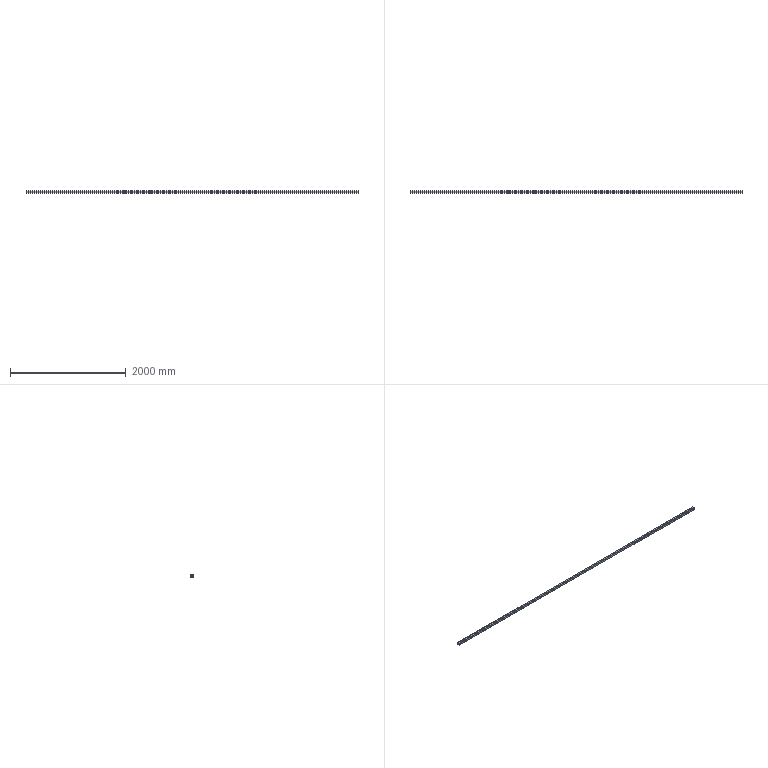Part | STEP file | SN10_003_008-04_TUBO_QUADRADO | 1 solid | 18 faces | box 5740 x 40 x 40 mm | volume 2415524 mm3 | plane 10 | cylinder 8 | commonest cylinder face diameters 6 x4 12 x4
STEP:
#1=CARTESIAN_POINT('',(0.,0.,0.));
#2=DIRECTION('',(0.,0.,1.));
#3=DIRECTION('',(1.,0.,0.));
#4=AXIS2_PLACEMENT_3D('',#1,#2,#3);
#5=CARTESIAN_POINT('',(0.,20.,14.));
#6=VERTEX_POINT('',#5);
#7=CARTESIAN_POINT('',(5740.,20.,14.));
#8=VERTEX_POINT('',#7);
#9=CARTESIAN_POINT('',(0.,20.,14.));
#10=DIRECTION('',(1.,0.,0.));
#11=VECTOR('',#10,1.);
#12=LINE('',#9,#11);
#13=CARTESIAN_POINT('',(2870.,14.,14.));
#14=DIRECTION('',(1.,0.,0.));
#15=DIRECTION('',(0.,1.,0.));
#16=AXIS2_PLACEMENT_3D('',#13,#14,#15);
#17=CYLINDRICAL_SURFACE('',#16,6.);
#18=CARTESIAN_POINT('',(0.,-2870.));
#19=DIRECTION('',(0.,1.));
#20=VECTOR('',#19,1.);
#21=LINE('',#18,#20);
#22=(GEOMETRIC_REPRESENTATION_CONTEXT(2)PARAMETRIC_REPRESENTATION_CONTEXT()REPRESENTATION_CONTEXT('',''));
#23=DEFINITIONAL_REPRESENTATION('',(#21),#22);
#24=PCURVE('',#17,#23);
#25=CARTESIAN_POINT('',(0.,20.,14.));
#26=DIRECTION('',(0.,-1.,0.));
#27=DIRECTION('',(0.,0.,-1.));
#28=AXIS2_PLACEMENT_3D('',#25,#26,#27);
#29=PLANE('',#28);
#30=CARTESIAN_POINT('',(0.,0.));
#31=DIRECTION('',(0.,1.));
#32=VECTOR('',#31,1.);
#33=LINE('',#30,#32);
#34=(GEOMETRIC_REPRESENTATION_CONTEXT(2)PARAMETRIC_REPRESENTATION_CONTEXT()REPRESENTATION_CONTEXT('',''));
#35=DEFINITIONAL_REPRESENTATION('',(#33),#34);
#36=PCURVE('',#29,#35);
#37=SURFACE_CURVE('',#12,(#24,#36),.PCURVE_S1.);
#38=EDGE_CURVE('',#6,#8,#37,.T.);
#39=ORIENTED_EDGE('',*,*,#38,.F.);
#40=CARTESIAN_POINT('',(0.,14.,20.));
#41=VERTEX_POINT('',#40);
#42=CARTESIAN_POINT('',(0.,14.,14.));
#43=DIRECTION('',(1.,0.,0.));
#44=DIRECTION('',(0.,1.,0.));
#45=AXIS2_PLACEMENT_3D('',#42,#43,#44);
#46=CIRCLE('',#45,6.);
#47=CARTESIAN_POINT('',(0.,-2870.));
#48=DIRECTION('',(1.,0.));
#49=VECTOR('',#48,1.);
#50=LINE('',#47,#49);
#51=(GEOMETRIC_REPRESENTATION_CONTEXT(2)PARAMETRIC_REPRESENTATION_CONTEXT()REPRESENTATION_CONTEXT('',''));
#52=DEFINITIONAL_REPRESENTATION('',(#50),#51);
#53=PCURVE('',#17,#52);
#54=CARTESIAN_POINT('',(0.,0.,0.));
#55=DIRECTION('',(1.,0.,0.));
#56=DIRECTION('',(0.,0.,-1.));
#57=AXIS2_PLACEMENT_3D('',#54,#55,#56);
#58=PLANE('',#57);
#59=CARTESIAN_POINT('',(-14.,14.));
#60=DIRECTION('',(0.,1.));
#61=AXIS2_PLACEMENT_2D('',#59,#60);
#62=CIRCLE('',#61,6.);
#63=(GEOMETRIC_REPRESENTATION_CONTEXT(2)PARAMETRIC_REPRESENTATION_CONTEXT()REPRESENTATION_CONTEXT('',''));
#64=DEFINITIONAL_REPRESENTATION('',(#62),#63);
#65=PCURVE('',#58,#64);
#66=SURFACE_CURVE('',#46,(#53,#65),.PCURVE_S1.);
#67=EDGE_CURVE('',#6,#41,#66,.T.);
#68=ORIENTED_EDGE('',*,*,#67,.T.);
#69=CARTESIAN_POINT('',(5740.,14.,20.));
#70=VERTEX_POINT('',#69);
#71=CARTESIAN_POINT('',(0.,14.,20.));
#72=DIRECTION('',(1.,0.,0.));
#73=VECTOR('',#72,1.);
#74=LINE('',#71,#73);
#75=CARTESIAN_POINT('',(1.571,-2870.));
#76=DIRECTION('',(0.,1.));
#77=VECTOR('',#76,1.);
#78=LINE('',#75,#77);
#79=(GEOMETRIC_REPRESENTATION_CONTEXT(2)PARAMETRIC_REPRESENTATION_CONTEXT()REPRESENTATION_CONTEXT('',''));
#80=DEFINITIONAL_REPRESENTATION('',(#78),#79);
#81=PCURVE('',#17,#80);
#82=CARTESIAN_POINT('',(0.,-14.,20.));
#83=DIRECTION('',(0.,0.,-1.));
#84=DIRECTION('',(-1.,0.,0.));
#85=AXIS2_PLACEMENT_3D('',#82,#83,#84);
#86=PLANE('',#85);
#87=CARTESIAN_POINT('',(0.,28.));
#88=DIRECTION('',(-1.,0.));
#89=VECTOR('',#88,1.);
#90=LINE('',#87,#89);
#91=(GEOMETRIC_REPRESENTATION_CONTEXT(2)PARAMETRIC_REPRESENTATION_CONTEXT()REPRESENTATION_CONTEXT('',''));
#92=DEFINITIONAL_REPRESENTATION('',(#90),#91);
#93=PCURVE('',#86,#92);
#94=SURFACE_CURVE('',#74,(#81,#93),.PCURVE_S1.);
#95=EDGE_CURVE('',#41,#70,#94,.T.);
#96=ORIENTED_EDGE('',*,*,#95,.T.);
#97=CARTESIAN_POINT('',(5740.,14.,14.));
#98=DIRECTION('',(1.,0.,0.));
#99=DIRECTION('',(0.,1.,0.));
#100=AXIS2_PLACEMENT_3D('',#97,#98,#99);
#101=CIRCLE('',#100,6.);
#102=CARTESIAN_POINT('',(0.,2870.));
#103=DIRECTION('',(1.,0.));
#104=VECTOR('',#103,1.);
#105=LINE('',#102,#104);
#106=(GEOMETRIC_REPRESENTATION_CONTEXT(2)PARAMETRIC_REPRESENTATION_CONTEXT()REPRESENTATION_CONTEXT('',''));
#107=DEFINITIONAL_REPRESENTATION('',(#105),#106);
#108=PCURVE('',#17,#107);
#109=CARTESIAN_POINT('',(5740.,0.,0.));
#110=DIRECTION('',(1.,0.,0.));
#111=DIRECTION('',(0.,0.,-1.));
#112=AXIS2_PLACEMENT_3D('',#109,#110,#111);
#113=PLANE('',#112);
#114=CARTESIAN_POINT('',(-14.,14.));
#115=DIRECTION('',(0.,1.));
#116=AXIS2_PLACEMENT_2D('',#114,#115);
#117=CIRCLE('',#116,6.);
#118=(GEOMETRIC_REPRESENTATION_CONTEXT(2)PARAMETRIC_REPRESENTATION_CONTEXT()REPRESENTATION_CONTEXT('',''));
#119=DEFINITIONAL_REPRESENTATION('',(#117),#118);
#120=PCURVE('',#113,#119);
#121=SURFACE_CURVE('',#101,(#108,#120),.PCURVE_S1.);
#122=EDGE_CURVE('',#8,#70,#121,.T.);
#123=ORIENTED_EDGE('',*,*,#122,.F.);
#124=EDGE_LOOP('',(#39,#68,#96,#123));
#125=FACE_BOUND('',#124,.T.);
#126=ADVANCED_FACE('',(#125),#17,.T.);
#127=ORIENTED_EDGE('',*,*,#95,.F.);
#128=CARTESIAN_POINT('',(0.,-14.,20.));
#129=VERTEX_POINT('',#128);
#130=CARTESIAN_POINT('',(0.,-14.,20.));
#131=DIRECTION('',(0.,1.,0.));
#132=VECTOR('',#131,1.);
#133=LINE('',#130,#132);
#134=CARTESIAN_POINT('',(0.,0.));
#135=DIRECTION('',(0.,1.));
#136=VECTOR('',#135,1.);
#137=LINE('',#134,#136);
#138=(GEOMETRIC_REPRESENTATION_CONTEXT(2)PARAMETRIC_REPRESENTATION_CONTEXT()REPRESENTATION_CONTEXT('',''));
#139=DEFINITIONAL_REPRESENTATION('',(#137),#138);
#140=PCURVE('',#86,#139);
#141=CARTESIAN_POINT('',(-20.,-14.));
#142=DIRECTION('',(0.,1.));
#143=VECTOR('',#142,1.);
#144=LINE('',#141,#143);
#145=(GEOMETRIC_REPRESENTATION_CONTEXT(2)PARAMETRIC_REPRESENTATION_CONTEXT()REPRESENTATION_CONTEXT('',''));
#146=DEFINITIONAL_REPRESENTATION('',(#144),#145);
#147=PCURVE('',#58,#146);
#148=SURFACE_CURVE('',#133,(#140,#147),.PCURVE_S1.);
#149=EDGE_CURVE('',#129,#41,#148,.T.);
#150=ORIENTED_EDGE('',*,*,#149,.F.);
#151=CARTESIAN_POINT('',(5740.,-14.,20.));
#152=VERTEX_POINT('',#151);
#153=CARTESIAN_POINT('',(0.,-14.,20.));
#154=DIRECTION('',(1.,0.,0.));
#155=VECTOR('',#154,1.);
#156=LINE('',#153,#155);
#157=CARTESIAN_POINT('',(0.,0.));
#158=DIRECTION('',(-1.,0.));
#159=VECTOR('',#158,1.);
#160=LINE('',#157,#159);
#161=(GEOMETRIC_REPRESENTATION_CONTEXT(2)PARAMETRIC_REPRESENTATION_CONTEXT()REPRESENTATION_CONTEXT('',''));
#162=DEFINITIONAL_REPRESENTATION('',(#160),#161);
#163=PCURVE('',#86,#162);
#164=CARTESIAN_POINT('',(2870.,-14.,14.));
#165=DIRECTION('',(1.,0.,0.));
#166=DIRECTION('',(0.,0.,1.));
#167=AXIS2_PLACEMENT_3D('',#164,#165,#166);
#168=CYLINDRICAL_SURFACE('',#167,6.);
#169=CARTESIAN_POINT('',(0.,-2870.));
#170=DIRECTION('',(0.,1.));
#171=VECTOR('',#170,1.);
#172=LINE('',#169,#171);
#173=(GEOMETRIC_REPRESENTATION_CONTEXT(2)PARAMETRIC_REPRESENTATION_CONTEXT()REPRESENTATION_CONTEXT('',''));
#174=DEFINITIONAL_REPRESENTATION('',(#172),#173);
#175=PCURVE('',#168,#174);
#176=SURFACE_CURVE('',#156,(#163,#175),.PCURVE_S1.);
#177=EDGE_CURVE('',#129,#152,#176,.T.);
#178=ORIENTED_EDGE('',*,*,#177,.T.);
#179=CARTESIAN_POINT('',(5740.,-14.,20.));
#180=DIRECTION('',(0.,1.,0.));
#181=VECTOR('',#180,1.);
#182=LINE('',#179,#181);
#183=CARTESIAN_POINT('',(-5740.,0.));
#184=DIRECTION('',(0.,1.));
#185=VECTOR('',#184,1.);
#186=LINE('',#183,#185);
#187=(GEOMETRIC_REPRESENTATION_CONTEXT(2)PARAMETRIC_REPRESENTATION_CONTEXT()REPRESENTATION_CONTEXT('',''));
#188=DEFINITIONAL_REPRESENTATION('',(#186),#187);
#189=PCURVE('',#86,#188);
#190=CARTESIAN_POINT('',(-20.,-14.));
#191=DIRECTION('',(0.,1.));
#192=VECTOR('',#191,1.);
#193=LINE('',#190,#192);
#194=(GEOMETRIC_REPRESENTATION_CONTEXT(2)PARAMETRIC_REPRESENTATION_CONTEXT()REPRESENTATION_CONTEXT('',''));
#195=DEFINITIONAL_REPRESENTATION('',(#193),#194);
#196=PCURVE('',#113,#195);
#197=SURFACE_CURVE('',#182,(#189,#196),.PCURVE_S1.);
#198=EDGE_CURVE('',#152,#70,#197,.T.);
#199=ORIENTED_EDGE('',*,*,#198,.T.);
#200=EDGE_LOOP('',(#127,#150,#178,#199));
#201=FACE_BOUND('',#200,.T.);
#202=ADVANCED_FACE('',(#201),#86,.F.);
#203=ORIENTED_EDGE('',*,*,#177,.F.);
#204=CARTESIAN_POINT('',(0.,-20.,14.));
#205=VERTEX_POINT('',#204);
#206=CARTESIAN_POINT('',(0.,-14.,14.));
#207=DIRECTION('',(1.,0.,0.));
#208=DIRECTION('',(0.,1.,0.));
#209=AXIS2_PLACEMENT_3D('',#206,#207,#208);
#210=CIRCLE('',#209,6.);
#211=CARTESIAN_POINT('',(-1.571,-2870.));
#212=DIRECTION('',(1.,0.));
#213=VECTOR('',#212,1.);
#214=LINE('',#211,#213);
#215=(GEOMETRIC_REPRESENTATION_CONTEXT(2)PARAMETRIC_REPRESENTATION_CONTEXT()REPRESENTATION_CONTEXT('',''));
#216=DEFINITIONAL_REPRESENTATION('',(#214),#215);
#217=PCURVE('',#168,#216);
#218=CARTESIAN_POINT('',(-14.,-14.));
#219=DIRECTION('',(0.,1.));
#220=AXIS2_PLACEMENT_2D('',#218,#219);
#221=CIRCLE('',#220,6.);
#222=(GEOMETRIC_REPRESENTATION_CONTEXT(2)PARAMETRIC_REPRESENTATION_CONTEXT()REPRESENTATION_CONTEXT('',''));
#223=DEFINITIONAL_REPRESENTATION('',(#221),#222);
#224=PCURVE('',#58,#223);
#225=SURFACE_CURVE('',#210,(#217,#224),.PCURVE_S1.);
#226=EDGE_CURVE('',#129,#205,#225,.T.);
#227=ORIENTED_EDGE('',*,*,#226,.T.);
#228=CARTESIAN_POINT('',(5740.,-20.,14.));
#229=VERTEX_POINT('',#228);
#230=CARTESIAN_POINT('',(0.,-20.,14.));
#231=DIRECTION('',(1.,0.,0.));
#232=VECTOR('',#231,1.);
#233=LINE('',#230,#232);
#234=CARTESIAN_POINT('',(1.571,-2870.));
#235=DIRECTION('',(0.,1.));
#236=VECTOR('',#235,1.);
#237=LINE('',#234,#236);
#238=(GEOMETRIC_REPRESENTATION_CONTEXT(2)PARAMETRIC_REPRESENTATION_CONTEXT()REPRESENTATION_CONTEXT('',''));
#239=DEFINITIONAL_REPRESENTATION('',(#237),#238);
#240=PCURVE('',#168,#239);
#241=CARTESIAN_POINT('',(0.,-20.,-14.));
#242=DIRECTION('',(0.,1.,0.));
#243=DIRECTION('',(0.,0.,1.));
#244=AXIS2_PLACEMENT_3D('',#241,#242,#243);
#245=PLANE('',#244);
#246=CARTESIAN_POINT('',(28.,0.));
#247=DIRECTION('',(0.,1.));
#248=VECTOR('',#247,1.);
#249=LINE('',#246,#248);
#250=(GEOMETRIC_REPRESENTATION_CONTEXT(2)PARAMETRIC_REPRESENTATION_CONTEXT()REPRESENTATION_CONTEXT('',''));
#251=DEFINITIONAL_REPRESENTATION('',(#249),#250);
#252=PCURVE('',#245,#251);
#253=SURFACE_CURVE('',#233,(#240,#252),.PCURVE_S1.);
#254=EDGE_CURVE('',#205,#229,#253,.T.);
#255=ORIENTED_EDGE('',*,*,#254,.T.);
#256=CARTESIAN_POINT('',(5740.,-14.,14.));
#257=DIRECTION('',(1.,0.,0.));
#258=DIRECTION('',(0.,1.,0.));
#259=AXIS2_PLACEMENT_3D('',#256,#257,#258);
#260=CIRCLE('',#259,6.);
#261=CARTESIAN_POINT('',(-1.571,2870.));
#262=DIRECTION('',(1.,0.));
#263=VECTOR('',#262,1.);
#264=LINE('',#261,#263);
#265=(GEOMETRIC_REPRESENTATION_CONTEXT(2)PARAMETRIC_REPRESENTATION_CONTEXT()REPRESENTATION_CONTEXT('',''));
#266=DEFINITIONAL_REPRESENTATION('',(#264),#265);
#267=PCURVE('',#168,#266);
#268=CARTESIAN_POINT('',(-14.,-14.));
#269=DIRECTION('',(0.,1.));
#270=AXIS2_PLACEMENT_2D('',#268,#269);
#271=CIRCLE('',#270,6.);
#272=(GEOMETRIC_REPRESENTATION_CONTEXT(2)PARAMETRIC_REPRESENTATION_CONTEXT()REPRESENTATION_CONTEXT('',''));
#273=DEFINITIONAL_REPRESENTATION('',(#271),#272);
#274=PCURVE('',#113,#273);
#275=SURFACE_CURVE('',#260,(#267,#274),.PCURVE_S1.);
#276=EDGE_CURVE('',#152,#229,#275,.T.);
#277=ORIENTED_EDGE('',*,*,#276,.F.);
#278=EDGE_LOOP('',(#203,#227,#255,#277));
#279=FACE_BOUND('',#278,.T.);
#280=ADVANCED_FACE('',(#279),#168,.T.);
#281=ORIENTED_EDGE('',*,*,#254,.F.);
#282=CARTESIAN_POINT('',(0.,-20.,-14.));
#283=VERTEX_POINT('',#282);
#284=CARTESIAN_POINT('',(0.,-20.,-14.));
#285=DIRECTION('',(0.,0.,1.));
#286=VECTOR('',#285,1.);
#287=LINE('',#284,#286);
#288=CARTESIAN_POINT('',(0.,0.));
#289=DIRECTION('',(1.,0.));
#290=VECTOR('',#289,1.);
#291=LINE('',#288,#290);
#292=(GEOMETRIC_REPRESENTATION_CONTEXT(2)PARAMETRIC_REPRESENTATION_CONTEXT()REPRESENTATION_CONTEXT('',''));
#293=DEFINITIONAL_REPRESENTATION('',(#291),#292);
#294=PCURVE('',#245,#293);
#295=CARTESIAN_POINT('',(14.,-20.));
#296=DIRECTION('',(-1.,0.));
#297=VECTOR('',#296,1.);
#298=LINE('',#295,#297);
#299=(GEOMETRIC_REPRESENTATION_CONTEXT(2)PARAMETRIC_REPRESENTATION_CONTEXT()REPRESENTATION_CONTEXT('',''));
#300=DEFINITIONAL_REPRESENTATION('',(#298),#299);
#301=PCURVE('',#58,#300);
#302=SURFACE_CURVE('',#287,(#294,#301),.PCURVE_S1.);
#303=EDGE_CURVE('',#283,#205,#302,.T.);
#304=ORIENTED_EDGE('',*,*,#303,.F.);
#305=CARTESIAN_POINT('',(5740.,-20.,-14.));
#306=VERTEX_POINT('',#305);
#307=CARTESIAN_POINT('',(0.,-20.,-14.));
#308=DIRECTION('',(1.,0.,0.));
#309=VECTOR('',#308,1.);
#310=LINE('',#307,#309);
#311=CARTESIAN_POINT('',(0.,0.));
#312=DIRECTION('',(0.,1.));
#313=VECTOR('',#312,1.);
#314=LINE('',#311,#313);
#315=(GEOMETRIC_REPRESENTATION_CONTEXT(2)PARAMETRIC_REPRESENTATION_CONTEXT()REPRESENTATION_CONTEXT('',''));
#316=DEFINITIONAL_REPRESENTATION('',(#314),#315);
#317=PCURVE('',#245,#316);
#318=CARTESIAN_POINT('',(2870.,-14.,-14.));
#319=DIRECTION('',(1.,0.,0.));
#320=DIRECTION('',(0.,-1.,0.));
#321=AXIS2_PLACEMENT_3D('',#318,#319,#320);
#322=CYLINDRICAL_SURFACE('',#321,6.);
#323=CARTESIAN_POINT('',(0.,-2870.));
#324=DIRECTION('',(0.,1.));
#325=VECTOR('',#324,1.);
#326=LINE('',#323,#325);
#327=(GEOMETRIC_REPRESENTATION_CONTEXT(2)PARAMETRIC_REPRESENTATION_CONTEXT()REPRESENTATION_CONTEXT('',''));
#328=DEFINITIONAL_REPRESENTATION('',(#326),#327);
#329=PCURVE('',#322,#328);
#330=SURFACE_CURVE('',#310,(#317,#329),.PCURVE_S1.);
#331=EDGE_CURVE('',#283,#306,#330,.T.);
#332=ORIENTED_EDGE('',*,*,#331,.T.);
#333=CARTESIAN_POINT('',(5740.,-20.,-14.));
#334=DIRECTION('',(0.,0.,1.));
#335=VECTOR('',#334,1.);
#336=LINE('',#333,#335);
#337=CARTESIAN_POINT('',(0.,5740.));
#338=DIRECTION('',(1.,0.));
#339=VECTOR('',#338,1.);
#340=LINE('',#337,#339);
#341=(GEOMETRIC_REPRESENTATION_CONTEXT(2)PARAMETRIC_REPRESENTATION_CONTEXT()REPRESENTATION_CONTEXT('',''));
#342=DEFINITIONAL_REPRESENTATION('',(#340),#341);
#343=PCURVE('',#245,#342);
#344=CARTESIAN_POINT('',(14.,-20.));
#345=DIRECTION('',(-1.,0.));
#346=VECTOR('',#345,1.);
#347=LINE('',#344,#346);
#348=(GEOMETRIC_REPRESENTATION_CONTEXT(2)PARAMETRIC_REPRESENTATION_CONTEXT()REPRESENTATION_CONTEXT('',''));
#349=DEFINITIONAL_REPRESENTATION('',(#347),#348);
#350=PCURVE('',#113,#349);
#351=SURFACE_CURVE('',#336,(#343,#350),.PCURVE_S1.);
#352=EDGE_CURVE('',#306,#229,#351,.T.);
#353=ORIENTED_EDGE('',*,*,#352,.T.);
#354=EDGE_LOOP('',(#281,#304,#332,#353));
#355=FACE_BOUND('',#354,.T.);
#356=ADVANCED_FACE('',(#355),#245,.F.);
#357=ORIENTED_EDGE('',*,*,#331,.F.);
#358=CARTESIAN_POINT('',(0.,-14.,-20.));
#359=VERTEX_POINT('',#358);
#360=CARTESIAN_POINT('',(0.,-14.,-14.));
#361=DIRECTION('',(1.,0.,0.));
#362=DIRECTION('',(0.,1.,0.));
#363=AXIS2_PLACEMENT_3D('',#360,#361,#362);
#364=CIRCLE('',#363,6.);
#365=CARTESIAN_POINT('',(-3.142,-2870.));
#366=DIRECTION('',(1.,0.));
#367=VECTOR('',#366,1.);
#368=LINE('',#365,#367);
#369=(GEOMETRIC_REPRESENTATION_CONTEXT(2)PARAMETRIC_REPRESENTATION_CONTEXT()REPRESENTATION_CONTEXT('',''));
#370=DEFINITIONAL_REPRESENTATION('',(#368),#369);
#371=PCURVE('',#322,#370);
#372=CARTESIAN_POINT('',(14.,-14.));
#373=DIRECTION('',(0.,1.));
#374=AXIS2_PLACEMENT_2D('',#372,#373);
#375=CIRCLE('',#374,6.);
#376=(GEOMETRIC_REPRESENTATION_CONTEXT(2)PARAMETRIC_REPRESENTATION_CONTEXT()REPRESENTATION_CONTEXT('',''));
#377=DEFINITIONAL_REPRESENTATION('',(#375),#376);
#378=PCURVE('',#58,#377);
#379=SURFACE_CURVE('',#364,(#371,#378),.PCURVE_S1.);
#380=EDGE_CURVE('',#283,#359,#379,.T.);
#381=ORIENTED_EDGE('',*,*,#380,.T.);
#382=CARTESIAN_POINT('',(5740.,-14.,-20.));
#383=VERTEX_POINT('',#382);
#384=CARTESIAN_POINT('',(0.,-14.,-20.));
#385=DIRECTION('',(1.,0.,0.));
#386=VECTOR('',#385,1.);
#387=LINE('',#384,#386);
#388=CARTESIAN_POINT('',(1.571,-2870.));
#389=DIRECTION('',(0.,1.));
#390=VECTOR('',#389,1.);
#391=LINE('',#388,#390);
#392=(GEOMETRIC_REPRESENTATION_CONTEXT(2)PARAMETRIC_REPRESENTATION_CONTEXT()REPRESENTATION_CONTEXT('',''));
#393=DEFINITIONAL_REPRESENTATION('',(#391),#392);
#394=PCURVE('',#322,#393);
#395=CARTESIAN_POINT('',(0.,14.,-20.));
#396=DIRECTION('',(0.,0.,1.));
#397=DIRECTION('',(1.,0.,0.));
#398=AXIS2_PLACEMENT_3D('',#395,#396,#397);
#399=PLANE('',#398);
#400=CARTESIAN_POINT('',(0.,-28.));
#401=DIRECTION('',(1.,0.));
#402=VECTOR('',#401,1.);
#403=LINE('',#400,#402);
#404=(GEOMETRIC_REPRESENTATION_CONTEXT(2)PARAMETRIC_REPRESENTATION_CONTEXT()REPRESENTATION_CONTEXT('',''));
#405=DEFINITIONAL_REPRESENTATION('',(#403),#404);
#406=PCURVE('',#399,#405);
#407=SURFACE_CURVE('',#387,(#394,#406),.PCURVE_S1.);
#408=EDGE_CURVE('',#359,#383,#407,.T.);
#409=ORIENTED_EDGE('',*,*,#408,.T.);
#410=CARTESIAN_POINT('',(5740.,-14.,-14.));
#411=DIRECTION('',(1.,0.,0.));
#412=DIRECTION('',(0.,1.,0.));
#413=AXIS2_PLACEMENT_3D('',#410,#411,#412);
#414=CIRCLE('',#413,6.);
#415=CARTESIAN_POINT('',(-3.142,2870.));
#416=DIRECTION('',(1.,0.));
#417=VECTOR('',#416,1.);
#418=LINE('',#415,#417);
#419=(GEOMETRIC_REPRESENTATION_CONTEXT(2)PARAMETRIC_REPRESENTATION_CONTEXT()REPRESENTATION_CONTEXT('',''));
#420=DEFINITIONAL_REPRESENTATION('',(#418),#419);
#421=PCURVE('',#322,#420);
#422=CARTESIAN_POINT('',(14.,-14.));
#423=DIRECTION('',(0.,1.));
#424=AXIS2_PLACEMENT_2D('',#422,#423);
#425=CIRCLE('',#424,6.);
#426=(GEOMETRIC_REPRESENTATION_CONTEXT(2)PARAMETRIC_REPRESENTATION_CONTEXT()REPRESENTATION_CONTEXT('',''));
#427=DEFINITIONAL_REPRESENTATION('',(#425),#426);
#428=PCURVE('',#113,#427);
#429=SURFACE_CURVE('',#414,(#421,#428),.PCURVE_S1.);
#430=EDGE_CURVE('',#306,#383,#429,.T.);
#431=ORIENTED_EDGE('',*,*,#430,.F.);
#432=EDGE_LOOP('',(#357,#381,#409,#431));
#433=FACE_BOUND('',#432,.T.);
#434=ADVANCED_FACE('',(#433),#322,.T.);
#435=ORIENTED_EDGE('',*,*,#408,.F.);
#436=CARTESIAN_POINT('',(0.,14.,-20.));
#437=VERTEX_POINT('',#436);
#438=CARTESIAN_POINT('',(0.,14.,-20.));
#439=DIRECTION('',(0.,-1.,0.));
#440=VECTOR('',#439,1.);
#441=LINE('',#438,#440);
#442=CARTESIAN_POINT('',(0.,0.));
#443=DIRECTION('',(0.,-1.));
#444=VECTOR('',#443,1.);
#445=LINE('',#442,#444);
#446=(GEOMETRIC_REPRESENTATION_CONTEXT(2)PARAMETRIC_REPRESENTATION_CONTEXT()REPRESENTATION_CONTEXT('',''));
#447=DEFINITIONAL_REPRESENTATION('',(#445),#446);
#448=PCURVE('',#399,#447);
#449=CARTESIAN_POINT('',(20.,14.));
#450=DIRECTION('',(0.,-1.));
#451=VECTOR('',#450,1.);
#452=LINE('',#449,#451);
#453=(GEOMETRIC_REPRESENTATION_CONTEXT(2)PARAMETRIC_REPRESENTATION_CONTEXT()REPRESENTATION_CONTEXT('',''));
#454=DEFINITIONAL_REPRESENTATION('',(#452),#453);
#455=PCURVE('',#58,#454);
#456=SURFACE_CURVE('',#441,(#448,#455),.PCURVE_S1.);
#457=EDGE_CURVE('',#437,#359,#456,.T.);
#458=ORIENTED_EDGE('',*,*,#457,.F.);
#459=CARTESIAN_POINT('',(5740.,14.,-20.));
#460=VERTEX_POINT('',#459);
#461=CARTESIAN_POINT('',(0.,14.,-20.));
#462=DIRECTION('',(1.,0.,0.));
#463=VECTOR('',#462,1.);
#464=LINE('',#461,#463);
#465=CARTESIAN_POINT('',(0.,0.));
#466=DIRECTION('',(1.,0.));
#467=VECTOR('',#466,1.);
#468=LINE('',#465,#467);
#469=(GEOMETRIC_REPRESENTATION_CONTEXT(2)PARAMETRIC_REPRESENTATION_CONTEXT()REPRESENTATION_CONTEXT('',''));
#470=DEFINITIONAL_REPRESENTATION('',(#468),#469);
#471=PCURVE('',#399,#470);
#472=CARTESIAN_POINT('',(2870.,14.,-14.));
#473=DIRECTION('',(1.,0.,0.));
#474=DIRECTION('',(0.,0.,-1.));
#475=AXIS2_PLACEMENT_3D('',#472,#473,#474);
#476=CYLINDRICAL_SURFACE('',#475,6.);
#477=CARTESIAN_POINT('',(0.,-2870.));
#478=DIRECTION('',(0.,1.));
#479=VECTOR('',#478,1.);
#480=LINE('',#477,#479);
#481=(GEOMETRIC_REPRESENTATION_CONTEXT(2)PARAMETRIC_REPRESENTATION_CONTEXT()REPRESENTATION_CONTEXT('',''));
#482=DEFINITIONAL_REPRESENTATION('',(#480),#481);
#483=PCURVE('',#476,#482);
#484=SURFACE_CURVE('',#464,(#471,#483),.PCURVE_S1.);
#485=EDGE_CURVE('',#437,#460,#484,.T.);
#486=ORIENTED_EDGE('',*,*,#485,.T.);
#487=CARTESIAN_POINT('',(5740.,14.,-20.));
#488=DIRECTION('',(0.,-1.,0.));
#489=VECTOR('',#488,1.);
#490=LINE('',#487,#489);
#491=CARTESIAN_POINT('',(5740.,0.));
#492=DIRECTION('',(0.,-1.));
#493=VECTOR('',#492,1.);
#494=LINE('',#491,#493);
#495=(GEOMETRIC_REPRESENTATION_CONTEXT(2)PARAMETRIC_REPRESENTATION_CONTEXT()REPRESENTATION_CONTEXT('',''));
#496=DEFINITIONAL_REPRESENTATION('',(#494),#495);
#497=PCURVE('',#399,#496);
#498=CARTESIAN_POINT('',(20.,14.));
#499=DIRECTION('',(0.,-1.));
#500=VECTOR('',#499,1.);
#501=LINE('',#498,#500);
#502=(GEOMETRIC_REPRESENTATION_CONTEXT(2)PARAMETRIC_REPRESENTATION_CONTEXT()REPRESENTATION_CONTEXT('',''));
#503=DEFINITIONAL_REPRESENTATION('',(#501),#502);
#504=PCURVE('',#113,#503);
#505=SURFACE_CURVE('',#490,(#497,#504),.PCURVE_S1.);
#506=EDGE_CURVE('',#460,#383,#505,.T.);
#507=ORIENTED_EDGE('',*,*,#506,.T.);
#508=EDGE_LOOP('',(#435,#458,#486,#507));
#509=FACE_BOUND('',#508,.T.);
#510=ADVANCED_FACE('',(#509),#399,.F.);
#511=ORIENTED_EDGE('',*,*,#485,.F.);
#512=CARTESIAN_POINT('',(0.,20.,-14.));
#513=VERTEX_POINT('',#512);
#514=CARTESIAN_POINT('',(0.,14.,-14.));
#515=DIRECTION('',(1.,0.,0.));
#516=DIRECTION('',(0.,1.,0.));
#517=AXIS2_PLACEMENT_3D('',#514,#515,#516);
#518=CIRCLE('',#517,6.);
#519=CARTESIAN_POINT('',(-4.712,-2870.));
#520=DIRECTION('',(1.,0.));
#521=VECTOR('',#520,1.);
#522=LINE('',#519,#521);
#523=(GEOMETRIC_REPRESENTATION_CONTEXT(2)PARAMETRIC_REPRESENTATION_CONTEXT()REPRESENTATION_CONTEXT('',''));
#524=DEFINITIONAL_REPRESENTATION('',(#522),#523);
#525=PCURVE('',#476,#524);
#526=CARTESIAN_POINT('',(14.,14.));
#527=DIRECTION('',(0.,1.));
#528=AXIS2_PLACEMENT_2D('',#526,#527);
#529=CIRCLE('',#528,6.);
#530=(GEOMETRIC_REPRESENTATION_CONTEXT(2)PARAMETRIC_REPRESENTATION_CONTEXT()REPRESENTATION_CONTEXT('',''));
#531=DEFINITIONAL_REPRESENTATION('',(#529),#530);
#532=PCURVE('',#58,#531);
#533=SURFACE_CURVE('',#518,(#525,#532),.PCURVE_S1.);
#534=EDGE_CURVE('',#437,#513,#533,.T.);
#535=ORIENTED_EDGE('',*,*,#534,.T.);
#536=CARTESIAN_POINT('',(5740.,20.,-14.));
#537=VERTEX_POINT('',#536);
#538=CARTESIAN_POINT('',(0.,20.,-14.));
#539=DIRECTION('',(1.,0.,0.));
#540=VECTOR('',#539,1.);
#541=LINE('',#538,#540);
#542=CARTESIAN_POINT('',(1.571,-2870.));
#543=DIRECTION('',(0.,1.));
#544=VECTOR('',#543,1.);
#545=LINE('',#542,#544);
#546=(GEOMETRIC_REPRESENTATION_CONTEXT(2)PARAMETRIC_REPRESENTATION_CONTEXT()REPRESENTATION_CONTEXT('',''));
#547=DEFINITIONAL_REPRESENTATION('',(#545),#546);
#548=PCURVE('',#476,#547);
#549=CARTESIAN_POINT('',(28.,0.));
#550=DIRECTION('',(0.,1.));
#551=VECTOR('',#550,1.);
#552=LINE('',#549,#551);
#553=(GEOMETRIC_REPRESENTATION_CONTEXT(2)PARAMETRIC_REPRESENTATION_CONTEXT()REPRESENTATION_CONTEXT('',''));
#554=DEFINITIONAL_REPRESENTATION('',(#552),#553);
#555=PCURVE('',#29,#554);
#556=SURFACE_CURVE('',#541,(#548,#555),.PCURVE_S1.);
#557=EDGE_CURVE('',#513,#537,#556,.T.);
#558=ORIENTED_EDGE('',*,*,#557,.T.);
#559=CARTESIAN_POINT('',(5740.,14.,-14.));
#560=DIRECTION('',(1.,0.,0.));
#561=DIRECTION('',(0.,1.,0.));
#562=AXIS2_PLACEMENT_3D('',#559,#560,#561);
#563=CIRCLE('',#562,6.);
#564=CARTESIAN_POINT('',(-4.712,2870.));
#565=DIRECTION('',(1.,0.));
#566=VECTOR('',#565,1.);
#567=LINE('',#564,#566);
#568=(GEOMETRIC_REPRESENTATION_CONTEXT(2)PARAMETRIC_REPRESENTATION_CONTEXT()REPRESENTATION_CONTEXT('',''));
#569=DEFINITIONAL_REPRESENTATION('',(#567),#568);
#570=PCURVE('',#476,#569);
#571=CARTESIAN_POINT('',(14.,14.));
#572=DIRECTION('',(0.,1.));
#573=AXIS2_PLACEMENT_2D('',#571,#572);
#574=CIRCLE('',#573,6.);
#575=(GEOMETRIC_REPRESENTATION_CONTEXT(2)PARAMETRIC_REPRESENTATION_CONTEXT()REPRESENTATION_CONTEXT('',''));
#576=DEFINITIONAL_REPRESENTATION('',(#574),#575);
#577=PCURVE('',#113,#576);
#578=SURFACE_CURVE('',#563,(#570,#577),.PCURVE_S1.);
#579=EDGE_CURVE('',#460,#537,#578,.T.);
#580=ORIENTED_EDGE('',*,*,#579,.F.);
#581=EDGE_LOOP('',(#511,#535,#558,#580));
#582=FACE_BOUND('',#581,.T.);
#583=ADVANCED_FACE('',(#582),#476,.T.);
#584=ORIENTED_EDGE('',*,*,#557,.F.);
#585=CARTESIAN_POINT('',(0.,20.,14.));
#586=DIRECTION('',(0.,0.,-1.));
#587=VECTOR('',#586,1.);
#588=LINE('',#585,#587);
#589=CARTESIAN_POINT('',(0.,0.));
#590=DIRECTION('',(1.,0.));
#591=VECTOR('',#590,1.);
#592=LINE('',#589,#591);
#593=(GEOMETRIC_REPRESENTATION_CONTEXT(2)PARAMETRIC_REPRESENTATION_CONTEXT()REPRESENTATION_CONTEXT('',''));
#594=DEFINITIONAL_REPRESENTATION('',(#592),#593);
#595=PCURVE('',#29,#594);
#596=CARTESIAN_POINT('',(-14.,20.));
#597=DIRECTION('',(1.,0.));
#598=VECTOR('',#597,1.);
#599=LINE('',#596,#598);
#600=(GEOMETRIC_REPRESENTATION_CONTEXT(2)PARAMETRIC_REPRESENTATION_CONTEXT()REPRESENTATION_CONTEXT('',''));
#601=DEFINITIONAL_REPRESENTATION('',(#599),#600);
#602=PCURVE('',#58,#601);
#603=SURFACE_CURVE('',#588,(#595,#602),.PCURVE_S1.);
#604=EDGE_CURVE('',#6,#513,#603,.T.);
#605=ORIENTED_EDGE('',*,*,#604,.F.);
#606=ORIENTED_EDGE('',*,*,#38,.T.);
#607=CARTESIAN_POINT('',(5740.,20.,14.));
#608=DIRECTION('',(0.,0.,-1.));
#609=VECTOR('',#608,1.);
#610=LINE('',#607,#609);
#611=CARTESIAN_POINT('',(0.,5740.));
#612=DIRECTION('',(1.,0.));
#613=VECTOR('',#612,1.);
#614=LINE('',#611,#613);
#615=(GEOMETRIC_REPRESENTATION_CONTEXT(2)PARAMETRIC_REPRESENTATION_CONTEXT()REPRESENTATION_CONTEXT('',''));
#616=DEFINITIONAL_REPRESENTATION('',(#614),#615);
#617=PCURVE('',#29,#616);
#618=CARTESIAN_POINT('',(-14.,20.));
#619=DIRECTION('',(1.,0.));
#620=VECTOR('',#619,1.);
#621=LINE('',#618,#620);
#622=(GEOMETRIC_REPRESENTATION_CONTEXT(2)PARAMETRIC_REPRESENTATION_CONTEXT()REPRESENTATION_CONTEXT('',''));
#623=DEFINITIONAL_REPRESENTATION('',(#621),#622);
#624=PCURVE('',#113,#623);
#625=SURFACE_CURVE('',#610,(#617,#624),.PCURVE_S1.);
#626=EDGE_CURVE('',#8,#537,#625,.T.);
#627=ORIENTED_EDGE('',*,*,#626,.T.);
#628=EDGE_LOOP('',(#584,#605,#606,#627));
#629=FACE_BOUND('',#628,.T.);
#630=ADVANCED_FACE('',(#629),#29,.F.);
#631=CARTESIAN_POINT('',(5740.,17.,14.));
#632=VERTEX_POINT('',#631);
#633=CARTESIAN_POINT('',(5740.,17.,-14.));
#634=VERTEX_POINT('',#633);
#635=CARTESIAN_POINT('',(5740.,17.,14.));
#636=DIRECTION('',(0.,0.,-1.));
#637=VECTOR('',#636,1.);
#638=LINE('',#635,#637);
#639=CARTESIAN_POINT('',(0.,17.,14.));
#640=DIRECTION('',(0.,-1.,0.));
#641=DIRECTION('',(0.,0.,-1.));
#642=AXIS2_PLACEMENT_3D('',#639,#640,#641);
#643=PLANE('',#642);
#644=CARTESIAN_POINT('',(0.,5740.));
#645=DIRECTION('',(1.,0.));
#646=VECTOR('',#645,1.);
#647=LINE('',#644,#646);
#648=(GEOMETRIC_REPRESENTATION_CONTEXT(2)PARAMETRIC_REPRESENTATION_CONTEXT()REPRESENTATION_CONTEXT('',''));
#649=DEFINITIONAL_REPRESENTATION('',(#647),#648);
#650=PCURVE('',#643,#649);
#651=CARTESIAN_POINT('',(-14.,17.));
#652=DIRECTION('',(1.,0.));
#653=VECTOR('',#652,1.);
#654=LINE('',#651,#653);
#655=(GEOMETRIC_REPRESENTATION_CONTEXT(2)PARAMETRIC_REPRESENTATION_CONTEXT()REPRESENTATION_CONTEXT('',''));
#656=DEFINITIONAL_REPRESENTATION('',(#654),#655);
#657=PCURVE('',#113,#656);
#658=SURFACE_CURVE('',#638,(#650,#657),.PCURVE_S1.);
#659=EDGE_CURVE('',#632,#634,#658,.T.);
#660=ORIENTED_EDGE('',*,*,#659,.F.);
#661=CARTESIAN_POINT('',(0.,17.,14.));
#662=VERTEX_POINT('',#661);
#663=CARTESIAN_POINT('',(0.,17.,14.));
#664=DIRECTION('',(1.,0.,0.));
#665=VECTOR('',#664,1.);
#666=LINE('',#663,#665);
#667=CARTESIAN_POINT('',(0.,0.));
#668=DIRECTION('',(0.,1.));
#669=VECTOR('',#668,1.);
#670=LINE('',#667,#669);
#671=(GEOMETRIC_REPRESENTATION_CONTEXT(2)PARAMETRIC_REPRESENTATION_CONTEXT()REPRESENTATION_CONTEXT('',''));
#672=DEFINITIONAL_REPRESENTATION('',(#670),#671);
#673=PCURVE('',#643,#672);
#674=CARTESIAN_POINT('',(2870.,14.,14.));
#675=DIRECTION('',(1.,0.,0.));
#676=DIRECTION('',(0.,1.,0.));
#677=AXIS2_PLACEMENT_3D('',#674,#675,#676);
#678=CYLINDRICAL_SURFACE('',#677,3.);
#679=CARTESIAN_POINT('',(0.,-2870.));
#680=DIRECTION('',(0.,1.));
#681=VECTOR('',#680,1.);
#682=LINE('',#679,#681);
#683=(GEOMETRIC_REPRESENTATION_CONTEXT(2)PARAMETRIC_REPRESENTATION_CONTEXT()REPRESENTATION_CONTEXT('',''));
#684=DEFINITIONAL_REPRESENTATION('',(#682),#683);
#685=PCURVE('',#678,#684);
#686=SURFACE_CURVE('',#666,(#673,#685),.PCURVE_S1.);
#687=EDGE_CURVE('',#662,#632,#686,.T.);
#688=ORIENTED_EDGE('',*,*,#687,.F.);
#689=CARTESIAN_POINT('',(0.,17.,-14.));
#690=VERTEX_POINT('',#689);
#691=CARTESIAN_POINT('',(0.,17.,14.));
#692=DIRECTION('',(0.,0.,-1.));
#693=VECTOR('',#692,1.);
#694=LINE('',#691,#693);
#695=CARTESIAN_POINT('',(0.,0.));
#696=DIRECTION('',(1.,0.));
#697=VECTOR('',#696,1.);
#698=LINE('',#695,#697);
#699=(GEOMETRIC_REPRESENTATION_CONTEXT(2)PARAMETRIC_REPRESENTATION_CONTEXT()REPRESENTATION_CONTEXT('',''));
#700=DEFINITIONAL_REPRESENTATION('',(#698),#699);
#701=PCURVE('',#643,#700);
#702=CARTESIAN_POINT('',(-14.,17.));
#703=DIRECTION('',(1.,0.));
#704=VECTOR('',#703,1.);
#705=LINE('',#702,#704);
#706=(GEOMETRIC_REPRESENTATION_CONTEXT(2)PARAMETRIC_REPRESENTATION_CONTEXT()REPRESENTATION_CONTEXT('',''));
#707=DEFINITIONAL_REPRESENTATION('',(#705),#706);
#708=PCURVE('',#58,#707);
#709=SURFACE_CURVE('',#694,(#701,#708),.PCURVE_S1.);
#710=EDGE_CURVE('',#662,#690,#709,.T.);
#711=ORIENTED_EDGE('',*,*,#710,.T.);
#712=CARTESIAN_POINT('',(0.,17.,-14.));
#713=DIRECTION('',(1.,0.,0.));
#714=VECTOR('',#713,1.);
#715=LINE('',#712,#714);
#716=CARTESIAN_POINT('',(28.,0.));
#717=DIRECTION('',(0.,1.));
#718=VECTOR('',#717,1.);
#719=LINE('',#716,#718);
#720=(GEOMETRIC_REPRESENTATION_CONTEXT(2)PARAMETRIC_REPRESENTATION_CONTEXT()REPRESENTATION_CONTEXT('',''));
#721=DEFINITIONAL_REPRESENTATION('',(#719),#720);
#722=PCURVE('',#643,#721);
#723=CARTESIAN_POINT('',(2870.,14.,-14.));
#724=DIRECTION('',(1.,0.,0.));
#725=DIRECTION('',(0.,0.,-1.));
#726=AXIS2_PLACEMENT_3D('',#723,#724,#725);
#727=CYLINDRICAL_SURFACE('',#726,3.);
#728=CARTESIAN_POINT('',(1.571,-2870.));
#729=DIRECTION('',(0.,1.));
#730=VECTOR('',#729,1.);
#731=LINE('',#728,#730);
#732=(GEOMETRIC_REPRESENTATION_CONTEXT(2)PARAMETRIC_REPRESENTATION_CONTEXT()REPRESENTATION_CONTEXT('',''));
#733=DEFINITIONAL_REPRESENTATION('',(#731),#732);
#734=PCURVE('',#727,#733);
#735=SURFACE_CURVE('',#715,(#722,#734),.PCURVE_S1.);
#736=EDGE_CURVE('',#690,#634,#735,.T.);
#737=ORIENTED_EDGE('',*,*,#736,.T.);
#738=EDGE_LOOP('',(#660,#688,#711,#737));
#739=FACE_BOUND('',#738,.T.);
#740=ADVANCED_FACE('',(#739),#643,.T.);
#741=CARTESIAN_POINT('',(0.,14.,-17.));
#742=VERTEX_POINT('',#741);
#743=CARTESIAN_POINT('',(5740.,14.,-17.));
#744=VERTEX_POINT('',#743);
#745=CARTESIAN_POINT('',(0.,14.,-17.));
#746=DIRECTION('',(1.,0.,0.));
#747=VECTOR('',#746,1.);
#748=LINE('',#745,#747);
#749=CARTESIAN_POINT('',(0.,-2870.));
#750=DIRECTION('',(0.,1.));
#751=VECTOR('',#750,1.);
#752=LINE('',#749,#751);
#753=(GEOMETRIC_REPRESENTATION_CONTEXT(2)PARAMETRIC_REPRESENTATION_CONTEXT()REPRESENTATION_CONTEXT('',''));
#754=DEFINITIONAL_REPRESENTATION('',(#752),#753);
#755=PCURVE('',#727,#754);
#756=CARTESIAN_POINT('',(0.,14.,-17.));
#757=DIRECTION('',(0.,0.,1.));
#758=DIRECTION('',(1.,0.,0.));
#759=AXIS2_PLACEMENT_3D('',#756,#757,#758);
#760=PLANE('',#759);
#761=CARTESIAN_POINT('',(0.,0.));
#762=DIRECTION('',(1.,0.));
#763=VECTOR('',#762,1.);
#764=LINE('',#761,#763);
#765=(GEOMETRIC_REPRESENTATION_CONTEXT(2)PARAMETRIC_REPRESENTATION_CONTEXT()REPRESENTATION_CONTEXT('',''));
#766=DEFINITIONAL_REPRESENTATION('',(#764),#765);
#767=PCURVE('',#760,#766);
#768=SURFACE_CURVE('',#748,(#755,#767),.PCURVE_S1.);
#769=EDGE_CURVE('',#742,#744,#768,.T.);
#770=ORIENTED_EDGE('',*,*,#769,.F.);
#771=CARTESIAN_POINT('',(0.,14.,-14.));
#772=DIRECTION('',(1.,0.,0.));
#773=DIRECTION('',(0.,1.,0.));
#774=AXIS2_PLACEMENT_3D('',#771,#772,#773);
#775=CIRCLE('',#774,3.);
#776=CARTESIAN_POINT('',(-4.712,-2870.));
#777=DIRECTION('',(1.,0.));
#778=VECTOR('',#777,1.);
#779=LINE('',#776,#778);
#780=(GEOMETRIC_REPRESENTATION_CONTEXT(2)PARAMETRIC_REPRESENTATION_CONTEXT()REPRESENTATION_CONTEXT('',''));
#781=DEFINITIONAL_REPRESENTATION('',(#779),#780);
#782=PCURVE('',#727,#781);
#783=CARTESIAN_POINT('',(14.,14.));
#784=DIRECTION('',(0.,1.));
#785=AXIS2_PLACEMENT_2D('',#783,#784);
#786=CIRCLE('',#785,3.);
#787=(GEOMETRIC_REPRESENTATION_CONTEXT(2)PARAMETRIC_REPRESENTATION_CONTEXT()REPRESENTATION_CONTEXT('',''));
#788=DEFINITIONAL_REPRESENTATION('',(#786),#787);
#789=PCURVE('',#58,#788);
#790=SURFACE_CURVE('',#775,(#782,#789),.PCURVE_S1.);
#791=EDGE_CURVE('',#742,#690,#790,.T.);
#792=ORIENTED_EDGE('',*,*,#791,.T.);
#793=ORIENTED_EDGE('',*,*,#736,.T.);
#794=CARTESIAN_POINT('',(5740.,14.,-14.));
#795=DIRECTION('',(1.,0.,0.));
#796=DIRECTION('',(0.,1.,0.));
#797=AXIS2_PLACEMENT_3D('',#794,#795,#796);
#798=CIRCLE('',#797,3.);
#799=CARTESIAN_POINT('',(-4.712,2870.));
#800=DIRECTION('',(1.,0.));
#801=VECTOR('',#800,1.);
#802=LINE('',#799,#801);
#803=(GEOMETRIC_REPRESENTATION_CONTEXT(2)PARAMETRIC_REPRESENTATION_CONTEXT()REPRESENTATION_CONTEXT('',''));
#804=DEFINITIONAL_REPRESENTATION('',(#802),#803);
#805=PCURVE('',#727,#804);
#806=CARTESIAN_POINT('',(14.,14.));
#807=DIRECTION('',(0.,1.));
#808=AXIS2_PLACEMENT_2D('',#806,#807);
#809=CIRCLE('',#808,3.);
#810=(GEOMETRIC_REPRESENTATION_CONTEXT(2)PARAMETRIC_REPRESENTATION_CONTEXT()REPRESENTATION_CONTEXT('',''));
#811=DEFINITIONAL_REPRESENTATION('',(#809),#810);
#812=PCURVE('',#113,#811);
#813=SURFACE_CURVE('',#798,(#805,#812),.PCURVE_S1.);
#814=EDGE_CURVE('',#744,#634,#813,.T.);
#815=ORIENTED_EDGE('',*,*,#814,.F.);
#816=EDGE_LOOP('',(#770,#792,#793,#815));
#817=FACE_BOUND('',#816,.F.);
#818=ADVANCED_FACE('',(#817),#727,.F.);
#819=CARTESIAN_POINT('',(5740.,-14.,-17.));
#820=VERTEX_POINT('',#819);
#821=CARTESIAN_POINT('',(5740.,14.,-17.));
#822=DIRECTION('',(0.,-1.,0.));
#823=VECTOR('',#822,1.);
#824=LINE('',#821,#823);
#825=CARTESIAN_POINT('',(5740.,0.));
#826=DIRECTION('',(0.,-1.));
#827=VECTOR('',#826,1.);
#828=LINE('',#825,#827);
#829=(GEOMETRIC_REPRESENTATION_CONTEXT(2)PARAMETRIC_REPRESENTATION_CONTEXT()REPRESENTATION_CONTEXT('',''));
#830=DEFINITIONAL_REPRESENTATION('',(#828),#829);
#831=PCURVE('',#760,#830);
#832=CARTESIAN_POINT('',(17.,14.));
#833=DIRECTION('',(0.,-1.));
#834=VECTOR('',#833,1.);
#835=LINE('',#832,#834);
#836=(GEOMETRIC_REPRESENTATION_CONTEXT(2)PARAMETRIC_REPRESENTATION_CONTEXT()REPRESENTATION_CONTEXT('',''));
#837=DEFINITIONAL_REPRESENTATION('',(#835),#836);
#838=PCURVE('',#113,#837);
#839=SURFACE_CURVE('',#824,(#831,#838),.PCURVE_S1.);
#840=EDGE_CURVE('',#744,#820,#839,.T.);
#841=ORIENTED_EDGE('',*,*,#840,.F.);
#842=ORIENTED_EDGE('',*,*,#769,.F.);
#843=CARTESIAN_POINT('',(0.,-14.,-17.));
#844=VERTEX_POINT('',#843);
#845=CARTESIAN_POINT('',(0.,14.,-17.));
#846=DIRECTION('',(0.,-1.,0.));
#847=VECTOR('',#846,1.);
#848=LINE('',#845,#847);
#849=CARTESIAN_POINT('',(0.,0.));
#850=DIRECTION('',(0.,-1.));
#851=VECTOR('',#850,1.);
#852=LINE('',#849,#851);
#853=(GEOMETRIC_REPRESENTATION_CONTEXT(2)PARAMETRIC_REPRESENTATION_CONTEXT()REPRESENTATION_CONTEXT('',''));
#854=DEFINITIONAL_REPRESENTATION('',(#852),#853);
#855=PCURVE('',#760,#854);
#856=CARTESIAN_POINT('',(17.,14.));
#857=DIRECTION('',(0.,-1.));
#858=VECTOR('',#857,1.);
#859=LINE('',#856,#858);
#860=(GEOMETRIC_REPRESENTATION_CONTEXT(2)PARAMETRIC_REPRESENTATION_CONTEXT()REPRESENTATION_CONTEXT('',''));
#861=DEFINITIONAL_REPRESENTATION('',(#859),#860);
#862=PCURVE('',#58,#861);
#863=SURFACE_CURVE('',#848,(#855,#862),.PCURVE_S1.);
#864=EDGE_CURVE('',#742,#844,#863,.T.);
#865=ORIENTED_EDGE('',*,*,#864,.T.);
#866=CARTESIAN_POINT('',(0.,-14.,-17.));
#867=DIRECTION('',(1.,0.,0.));
#868=VECTOR('',#867,1.);
#869=LINE('',#866,#868);
#870=CARTESIAN_POINT('',(0.,-28.));
#871=DIRECTION('',(1.,0.));
#872=VECTOR('',#871,1.);
#873=LINE('',#870,#872);
#874=(GEOMETRIC_REPRESENTATION_CONTEXT(2)PARAMETRIC_REPRESENTATION_CONTEXT()REPRESENTATION_CONTEXT('',''));
#875=DEFINITIONAL_REPRESENTATION('',(#873),#874);
#876=PCURVE('',#760,#875);
#877=CARTESIAN_POINT('',(2870.,-14.,-14.));
#878=DIRECTION('',(1.,0.,0.));
#879=DIRECTION('',(0.,-1.,0.));
#880=AXIS2_PLACEMENT_3D('',#877,#878,#879);
#881=CYLINDRICAL_SURFACE('',#880,3.);
#882=CARTESIAN_POINT('',(1.571,-2870.));
#883=DIRECTION('',(0.,1.));
#884=VECTOR('',#883,1.);
#885=LINE('',#882,#884);
#886=(GEOMETRIC_REPRESENTATION_CONTEXT(2)PARAMETRIC_REPRESENTATION_CONTEXT()REPRESENTATION_CONTEXT('',''));
#887=DEFINITIONAL_REPRESENTATION('',(#885),#886);
#888=PCURVE('',#881,#887);
#889=SURFACE_CURVE('',#869,(#876,#888),.PCURVE_S1.);
#890=EDGE_CURVE('',#844,#820,#889,.T.);
#891=ORIENTED_EDGE('',*,*,#890,.T.);
#892=EDGE_LOOP('',(#841,#842,#865,#891));
#893=FACE_BOUND('',#892,.T.);
#894=ADVANCED_FACE('',(#893),#760,.T.);
#895=CARTESIAN_POINT('',(0.,-17.,-14.));
#896=VERTEX_POINT('',#895);
#897=CARTESIAN_POINT('',(5740.,-17.,-14.));
#898=VERTEX_POINT('',#897);
#899=CARTESIAN_POINT('',(0.,-17.,-14.));
#900=DIRECTION('',(1.,0.,0.));
#901=VECTOR('',#900,1.);
#902=LINE('',#899,#901);
#903=CARTESIAN_POINT('',(0.,-2870.));
#904=DIRECTION('',(0.,1.));
#905=VECTOR('',#904,1.);
#906=LINE('',#903,#905);
#907=(GEOMETRIC_REPRESENTATION_CONTEXT(2)PARAMETRIC_REPRESENTATION_CONTEXT()REPRESENTATION_CONTEXT('',''));
#908=DEFINITIONAL_REPRESENTATION('',(#906),#907);
#909=PCURVE('',#881,#908);
#910=CARTESIAN_POINT('',(0.,-17.,-14.));
#911=DIRECTION('',(0.,1.,0.));
#912=DIRECTION('',(0.,0.,1.));
#913=AXIS2_PLACEMENT_3D('',#910,#911,#912);
#914=PLANE('',#913);
#915=CARTESIAN_POINT('',(0.,0.));
#916=DIRECTION('',(0.,1.));
#917=VECTOR('',#916,1.);
#918=LINE('',#915,#917);
#919=(GEOMETRIC_REPRESENTATION_CONTEXT(2)PARAMETRIC_REPRESENTATION_CONTEXT()REPRESENTATION_CONTEXT('',''));
#920=DEFINITIONAL_REPRESENTATION('',(#918),#919);
#921=PCURVE('',#914,#920);
#922=SURFACE_CURVE('',#902,(#909,#921),.PCURVE_S1.);
#923=EDGE_CURVE('',#896,#898,#922,.T.);
#924=ORIENTED_EDGE('',*,*,#923,.F.);
#925=CARTESIAN_POINT('',(0.,-14.,-14.));
#926=DIRECTION('',(1.,0.,0.));
#927=DIRECTION('',(0.,1.,0.));
#928=AXIS2_PLACEMENT_3D('',#925,#926,#927);
#929=CIRCLE('',#928,3.);
#930=CARTESIAN_POINT('',(-3.142,-2870.));
#931=DIRECTION('',(1.,0.));
#932=VECTOR('',#931,1.);
#933=LINE('',#930,#932);
#934=(GEOMETRIC_REPRESENTATION_CONTEXT(2)PARAMETRIC_REPRESENTATION_CONTEXT()REPRESENTATION_CONTEXT('',''));
#935=DEFINITIONAL_REPRESENTATION('',(#933),#934);
#936=PCURVE('',#881,#935);
#937=CARTESIAN_POINT('',(14.,-14.));
#938=DIRECTION('',(0.,1.));
#939=AXIS2_PLACEMENT_2D('',#937,#938);
#940=CIRCLE('',#939,3.);
#941=(GEOMETRIC_REPRESENTATION_CONTEXT(2)PARAMETRIC_REPRESENTATION_CONTEXT()REPRESENTATION_CONTEXT('',''));
#942=DEFINITIONAL_REPRESENTATION('',(#940),#941);
#943=PCURVE('',#58,#942);
#944=SURFACE_CURVE('',#929,(#936,#943),.PCURVE_S1.);
#945=EDGE_CURVE('',#896,#844,#944,.T.);
#946=ORIENTED_EDGE('',*,*,#945,.T.);
#947=ORIENTED_EDGE('',*,*,#890,.T.);
#948=CARTESIAN_POINT('',(5740.,-14.,-14.));
#949=DIRECTION('',(1.,0.,0.));
#950=DIRECTION('',(0.,1.,0.));
#951=AXIS2_PLACEMENT_3D('',#948,#949,#950);
#952=CIRCLE('',#951,3.);
#953=CARTESIAN_POINT('',(-3.142,2870.));
#954=DIRECTION('',(1.,0.));
#955=VECTOR('',#954,1.);
#956=LINE('',#953,#955);
#957=(GEOMETRIC_REPRESENTATION_CONTEXT(2)PARAMETRIC_REPRESENTATION_CONTEXT()REPRESENTATION_CONTEXT('',''));
#958=DEFINITIONAL_REPRESENTATION('',(#956),#957);
#959=PCURVE('',#881,#958);
#960=CARTESIAN_POINT('',(14.,-14.));
#961=DIRECTION('',(0.,1.));
#962=AXIS2_PLACEMENT_2D('',#960,#961);
#963=CIRCLE('',#962,3.);
#964=(GEOMETRIC_REPRESENTATION_CONTEXT(2)PARAMETRIC_REPRESENTATION_CONTEXT()REPRESENTATION_CONTEXT('',''));
#965=DEFINITIONAL_REPRESENTATION('',(#963),#964);
#966=PCURVE('',#113,#965);
#967=SURFACE_CURVE('',#952,(#959,#966),.PCURVE_S1.);
#968=EDGE_CURVE('',#898,#820,#967,.T.);
#969=ORIENTED_EDGE('',*,*,#968,.F.);
#970=EDGE_LOOP('',(#924,#946,#947,#969));
#971=FACE_BOUND('',#970,.F.);
#972=ADVANCED_FACE('',(#971),#881,.F.);
#973=CARTESIAN_POINT('',(5740.,-17.,14.));
#974=VERTEX_POINT('',#973);
#975=CARTESIAN_POINT('',(5740.,-17.,-14.));
#976=DIRECTION('',(0.,0.,1.));
#977=VECTOR('',#976,1.);
#978=LINE('',#975,#977);
#979=CARTESIAN_POINT('',(0.,5740.));
#980=DIRECTION('',(1.,0.));
#981=VECTOR('',#980,1.);
#982=LINE('',#979,#981);
#983=(GEOMETRIC_REPRESENTATION_CONTEXT(2)PARAMETRIC_REPRESENTATION_CONTEXT()REPRESENTATION_CONTEXT('',''));
#984=DEFINITIONAL_REPRESENTATION('',(#982),#983);
#985=PCURVE('',#914,#984);
#986=CARTESIAN_POINT('',(14.,-17.));
#987=DIRECTION('',(-1.,0.));
#988=VECTOR('',#987,1.);
#989=LINE('',#986,#988);
#990=(GEOMETRIC_REPRESENTATION_CONTEXT(2)PARAMETRIC_REPRESENTATION_CONTEXT()REPRESENTATION_CONTEXT('',''));
#991=DEFINITIONAL_REPRESENTATION('',(#989),#990);
#992=PCURVE('',#113,#991);
#993=SURFACE_CURVE('',#978,(#985,#992),.PCURVE_S1.);
#994=EDGE_CURVE('',#898,#974,#993,.T.);
#995=ORIENTED_EDGE('',*,*,#994,.F.);
#996=ORIENTED_EDGE('',*,*,#923,.F.);
#997=CARTESIAN_POINT('',(0.,-17.,14.));
#998=VERTEX_POINT('',#997);
#999=CARTESIAN_POINT('',(0.,-17.,-14.));
#1000=DIRECTION('',(0.,0.,1.));
#1001=VECTOR('',#1000,1.);
#1002=LINE('',#999,#1001);
#1003=CARTESIAN_POINT('',(0.,0.));
#1004=DIRECTION('',(1.,0.));
#1005=VECTOR('',#1004,1.);
#1006=LINE('',#1003,#1005);
#1007=(GEOMETRIC_REPRESENTATION_CONTEXT(2)PARAMETRIC_REPRESENTATION_CONTEXT()REPRESENTATION_CONTEXT('',''));
#1008=DEFINITIONAL_REPRESENTATION('',(#1006),#1007);
#1009=PCURVE('',#914,#1008);
#1010=CARTESIAN_POINT('',(14.,-17.));
#1011=DIRECTION('',(-1.,0.));
#1012=VECTOR('',#1011,1.);
#1013=LINE('',#1010,#1012);
#1014=(GEOMETRIC_REPRESENTATION_CONTEXT(2)PARAMETRIC_REPRESENTATION_CONTEXT()REPRESENTATION_CONTEXT('',''));
#1015=DEFINITIONAL_REPRESENTATION('',(#1013),#1014);
#1016=PCURVE('',#58,#1015);
#1017=SURFACE_CURVE('',#1002,(#1009,#1016),.PCURVE_S1.);
#1018=EDGE_CURVE('',#896,#998,#1017,.T.);
#1019=ORIENTED_EDGE('',*,*,#1018,.T.);
#1020=CARTESIAN_POINT('',(0.,-17.,14.));
#1021=DIRECTION('',(1.,0.,0.));
#1022=VECTOR('',#1021,1.);
#1023=LINE('',#1020,#1022);
#1024=CARTESIAN_POINT('',(28.,0.));
#1025=DIRECTION('',(0.,1.));
#1026=VECTOR('',#1025,1.);
#1027=LINE('',#1024,#1026);
#1028=(GEOMETRIC_REPRESENTATION_CONTEXT(2)PARAMETRIC_REPRESENTATION_CONTEXT()REPRESENTATION_CONTEXT('',''));
#1029=DEFINITIONAL_REPRESENTATION('',(#1027),#1028);
#1030=PCURVE('',#914,#1029);
#1031=CARTESIAN_POINT('',(2870.,-14.,14.));
#1032=DIRECTION('',(1.,0.,0.));
#1033=DIRECTION('',(0.,0.,1.));
#1034=AXIS2_PLACEMENT_3D('',#1031,#1032,#1033);
#1035=CYLINDRICAL_SURFACE('',#1034,3.);
#1036=CARTESIAN_POINT('',(1.571,-2870.));
#1037=DIRECTION('',(0.,1.));
#1038=VECTOR('',#1037,1.);
#1039=LINE('',#1036,#1038);
#1040=(GEOMETRIC_REPRESENTATION_CONTEXT(2)PARAMETRIC_REPRESENTATION_CONTEXT()REPRESENTATION_CONTEXT('',''));
#1041=DEFINITIONAL_REPRESENTATION('',(#1039),#1040);
#1042=PCURVE('',#1035,#1041);
#1043=SURFACE_CURVE('',#1023,(#1030,#1042),.PCURVE_S1.);
#1044=EDGE_CURVE('',#998,#974,#1043,.T.);
#1045=ORIENTED_EDGE('',*,*,#1044,.T.);
#1046=EDGE_LOOP('',(#995,#996,#1019,#1045));
#1047=FACE_BOUND('',#1046,.T.);
#1048=ADVANCED_FACE('',(#1047),#914,.T.);
#1049=CARTESIAN_POINT('',(0.,-14.,17.));
#1050=VERTEX_POINT('',#1049);
#1051=CARTESIAN_POINT('',(5740.,-14.,17.));
#1052=VERTEX_POINT('',#1051);
#1053=CARTESIAN_POINT('',(0.,-14.,17.));
#1054=DIRECTION('',(1.,0.,0.));
#1055=VECTOR('',#1054,1.);
#1056=LINE('',#1053,#1055);
#1057=CARTESIAN_POINT('',(0.,-2870.));
#1058=DIRECTION('',(0.,1.));
#1059=VECTOR('',#1058,1.);
#1060=LINE('',#1057,#1059);
#1061=(GEOMETRIC_REPRESENTATION_CONTEXT(2)PARAMETRIC_REPRESENTATION_CONTEXT()REPRESENTATION_CONTEXT('',''));
#1062=DEFINITIONAL_REPRESENTATION('',(#1060),#1061);
#1063=PCURVE('',#1035,#1062);
#1064=CARTESIAN_POINT('',(0.,-14.,17.));
#1065=DIRECTION('',(0.,0.,-1.));
#1066=DIRECTION('',(-1.,0.,0.));
#1067=AXIS2_PLACEMENT_3D('',#1064,#1065,#1066);
#1068=PLANE('',#1067);
#1069=CARTESIAN_POINT('',(0.,0.));
#1070=DIRECTION('',(-1.,0.));
#1071=VECTOR('',#1070,1.);
#1072=LINE('',#1069,#1071);
#1073=(GEOMETRIC_REPRESENTATION_CONTEXT(2)PARAMETRIC_REPRESENTATION_CONTEXT()REPRESENTATION_CONTEXT('',''));
#1074=DEFINITIONAL_REPRESENTATION('',(#1072),#1073);
#1075=PCURVE('',#1068,#1074);
#1076=SURFACE_CURVE('',#1056,(#1063,#1075),.PCURVE_S1.);
#1077=EDGE_CURVE('',#1050,#1052,#1076,.T.);
#1078=ORIENTED_EDGE('',*,*,#1077,.F.);
#1079=CARTESIAN_POINT('',(0.,-14.,14.));
#1080=DIRECTION('',(1.,0.,0.));
#1081=DIRECTION('',(0.,1.,0.));
#1082=AXIS2_PLACEMENT_3D('',#1079,#1080,#1081);
#1083=CIRCLE('',#1082,3.);
#1084=CARTESIAN_POINT('',(-1.571,-2870.));
#1085=DIRECTION('',(1.,0.));
#1086=VECTOR('',#1085,1.);
#1087=LINE('',#1084,#1086);
#1088=(GEOMETRIC_REPRESENTATION_CONTEXT(2)PARAMETRIC_REPRESENTATION_CONTEXT()REPRESENTATION_CONTEXT('',''));
#1089=DEFINITIONAL_REPRESENTATION('',(#1087),#1088);
#1090=PCURVE('',#1035,#1089);
#1091=CARTESIAN_POINT('',(-14.,-14.));
#1092=DIRECTION('',(0.,1.));
#1093=AXIS2_PLACEMENT_2D('',#1091,#1092);
#1094=CIRCLE('',#1093,3.);
#1095=(GEOMETRIC_REPRESENTATION_CONTEXT(2)PARAMETRIC_REPRESENTATION_CONTEXT()REPRESENTATION_CONTEXT('',''));
#1096=DEFINITIONAL_REPRESENTATION('',(#1094),#1095);
#1097=PCURVE('',#58,#1096);
#1098=SURFACE_CURVE('',#1083,(#1090,#1097),.PCURVE_S1.);
#1099=EDGE_CURVE('',#1050,#998,#1098,.T.);
#1100=ORIENTED_EDGE('',*,*,#1099,.T.);
#1101=ORIENTED_EDGE('',*,*,#1044,.T.);
#1102=CARTESIAN_POINT('',(5740.,-14.,14.));
#1103=DIRECTION('',(1.,0.,0.));
#1104=DIRECTION('',(0.,1.,0.));
#1105=AXIS2_PLACEMENT_3D('',#1102,#1103,#1104);
#1106=CIRCLE('',#1105,3.);
#1107=CARTESIAN_POINT('',(-1.571,2870.));
#1108=DIRECTION('',(1.,0.));
#1109=VECTOR('',#1108,1.);
#1110=LINE('',#1107,#1109);
#1111=(GEOMETRIC_REPRESENTATION_CONTEXT(2)PARAMETRIC_REPRESENTATION_CONTEXT()REPRESENTATION_CONTEXT('',''));
#1112=DEFINITIONAL_REPRESENTATION('',(#1110),#1111);
#1113=PCURVE('',#1035,#1112);
#1114=CARTESIAN_POINT('',(-14.,-14.));
#1115=DIRECTION('',(0.,1.));
#1116=AXIS2_PLACEMENT_2D('',#1114,#1115);
#1117=CIRCLE('',#1116,3.);
#1118=(GEOMETRIC_REPRESENTATION_CONTEXT(2)PARAMETRIC_REPRESENTATION_CONTEXT()REPRESENTATION_CONTEXT('',''));
#1119=DEFINITIONAL_REPRESENTATION('',(#1117),#1118);
#1120=PCURVE('',#113,#1119);
#1121=SURFACE_CURVE('',#1106,(#1113,#1120),.PCURVE_S1.);
#1122=EDGE_CURVE('',#1052,#974,#1121,.T.);
#1123=ORIENTED_EDGE('',*,*,#1122,.F.);
#1124=EDGE_LOOP('',(#1078,#1100,#1101,#1123));
#1125=FACE_BOUND('',#1124,.F.);
#1126=ADVANCED_FACE('',(#1125),#1035,.F.);
#1127=CARTESIAN_POINT('',(5740.,14.,17.));
#1128=VERTEX_POINT('',#1127);
#1129=CARTESIAN_POINT('',(5740.,-14.,17.));
#1130=DIRECTION('',(0.,1.,0.));
#1131=VECTOR('',#1130,1.);
#1132=LINE('',#1129,#1131);
#1133=CARTESIAN_POINT('',(-5740.,0.));
#1134=DIRECTION('',(0.,1.));
#1135=VECTOR('',#1134,1.);
#1136=LINE('',#1133,#1135);
#1137=(GEOMETRIC_REPRESENTATION_CONTEXT(2)PARAMETRIC_REPRESENTATION_CONTEXT()REPRESENTATION_CONTEXT('',''));
#1138=DEFINITIONAL_REPRESENTATION('',(#1136),#1137);
#1139=PCURVE('',#1068,#1138);
#1140=CARTESIAN_POINT('',(-17.,-14.));
#1141=DIRECTION('',(0.,1.));
#1142=VECTOR('',#1141,1.);
#1143=LINE('',#1140,#1142);
#1144=(GEOMETRIC_REPRESENTATION_CONTEXT(2)PARAMETRIC_REPRESENTATION_CONTEXT()REPRESENTATION_CONTEXT('',''));
#1145=DEFINITIONAL_REPRESENTATION('',(#1143),#1144);
#1146=PCURVE('',#113,#1145);
#1147=SURFACE_CURVE('',#1132,(#1139,#1146),.PCURVE_S1.);
#1148=EDGE_CURVE('',#1052,#1128,#1147,.T.);
#1149=ORIENTED_EDGE('',*,*,#1148,.F.);
#1150=ORIENTED_EDGE('',*,*,#1077,.F.);
#1151=CARTESIAN_POINT('',(0.,14.,17.));
#1152=VERTEX_POINT('',#1151);
#1153=CARTESIAN_POINT('',(0.,-14.,17.));
#1154=DIRECTION('',(0.,1.,0.));
#1155=VECTOR('',#1154,1.);
#1156=LINE('',#1153,#1155);
#1157=CARTESIAN_POINT('',(0.,0.));
#1158=DIRECTION('',(0.,1.));
#1159=VECTOR('',#1158,1.);
#1160=LINE('',#1157,#1159);
#1161=(GEOMETRIC_REPRESENTATION_CONTEXT(2)PARAMETRIC_REPRESENTATION_CONTEXT()REPRESENTATION_CONTEXT('',''));
#1162=DEFINITIONAL_REPRESENTATION('',(#1160),#1161);
#1163=PCURVE('',#1068,#1162);
#1164=CARTESIAN_POINT('',(-17.,-14.));
#1165=DIRECTION('',(0.,1.));
#1166=VECTOR('',#1165,1.);
#1167=LINE('',#1164,#1166);
#1168=(GEOMETRIC_REPRESENTATION_CONTEXT(2)PARAMETRIC_REPRESENTATION_CONTEXT()REPRESENTATION_CONTEXT('',''));
#1169=DEFINITIONAL_REPRESENTATION('',(#1167),#1168);
#1170=PCURVE('',#58,#1169);
#1171=SURFACE_CURVE('',#1156,(#1163,#1170),.PCURVE_S1.);
#1172=EDGE_CURVE('',#1050,#1152,#1171,.T.);
#1173=ORIENTED_EDGE('',*,*,#1172,.T.);
#1174=CARTESIAN_POINT('',(0.,14.,17.));
#1175=DIRECTION('',(1.,0.,0.));
#1176=VECTOR('',#1175,1.);
#1177=LINE('',#1174,#1176);
#1178=CARTESIAN_POINT('',(0.,28.));
#1179=DIRECTION('',(-1.,0.));
#1180=VECTOR('',#1179,1.);
#1181=LINE('',#1178,#1180);
#1182=(GEOMETRIC_REPRESENTATION_CONTEXT(2)PARAMETRIC_REPRESENTATION_CONTEXT()REPRESENTATION_CONTEXT('',''));
#1183=DEFINITIONAL_REPRESENTATION('',(#1181),#1182);
#1184=PCURVE('',#1068,#1183);
#1185=CARTESIAN_POINT('',(1.571,-2870.));
#1186=DIRECTION('',(0.,1.));
#1187=VECTOR('',#1186,1.);
#1188=LINE('',#1185,#1187);
#1189=(GEOMETRIC_REPRESENTATION_CONTEXT(2)PARAMETRIC_REPRESENTATION_CONTEXT()REPRESENTATION_CONTEXT('',''));
#1190=DEFINITIONAL_REPRESENTATION('',(#1188),#1189);
#1191=PCURVE('',#678,#1190);
#1192=SURFACE_CURVE('',#1177,(#1184,#1191),.PCURVE_S1.);
#1193=EDGE_CURVE('',#1152,#1128,#1192,.T.);
#1194=ORIENTED_EDGE('',*,*,#1193,.T.);
#1195=EDGE_LOOP('',(#1149,#1150,#1173,#1194));
#1196=FACE_BOUND('',#1195,.T.);
#1197=ADVANCED_FACE('',(#1196),#1068,.T.);
#1198=ORIENTED_EDGE('',*,*,#687,.F.);
#1199=CARTESIAN_POINT('',(0.,14.,14.));
#1200=DIRECTION('',(1.,0.,0.));
#1201=DIRECTION('',(0.,1.,0.));
#1202=AXIS2_PLACEMENT_3D('',#1199,#1200,#1201);
#1203=CIRCLE('',#1202,3.);
#1204=CARTESIAN_POINT('',(0.,-2870.));
#1205=DIRECTION('',(1.,0.));
#1206=VECTOR('',#1205,1.);
#1207=LINE('',#1204,#1206);
#1208=(GEOMETRIC_REPRESENTATION_CONTEXT(2)PARAMETRIC_REPRESENTATION_CONTEXT()REPRESENTATION_CONTEXT('',''));
#1209=DEFINITIONAL_REPRESENTATION('',(#1207),#1208);
#1210=PCURVE('',#678,#1209);
#1211=CARTESIAN_POINT('',(-14.,14.));
#1212=DIRECTION('',(0.,1.));
#1213=AXIS2_PLACEMENT_2D('',#1211,#1212);
#1214=CIRCLE('',#1213,3.);
#1215=(GEOMETRIC_REPRESENTATION_CONTEXT(2)PARAMETRIC_REPRESENTATION_CONTEXT()REPRESENTATION_CONTEXT('',''));
#1216=DEFINITIONAL_REPRESENTATION('',(#1214),#1215);
#1217=PCURVE('',#58,#1216);
#1218=SURFACE_CURVE('',#1203,(#1210,#1217),.PCURVE_S1.);
#1219=EDGE_CURVE('',#662,#1152,#1218,.T.);
#1220=ORIENTED_EDGE('',*,*,#1219,.T.);
#1221=ORIENTED_EDGE('',*,*,#1193,.T.);
#1222=CARTESIAN_POINT('',(5740.,14.,14.));
#1223=DIRECTION('',(1.,0.,0.));
#1224=DIRECTION('',(0.,1.,0.));
#1225=AXIS2_PLACEMENT_3D('',#1222,#1223,#1224);
#1226=CIRCLE('',#1225,3.);
#1227=CARTESIAN_POINT('',(0.,2870.));
#1228=DIRECTION('',(1.,0.));
#1229=VECTOR('',#1228,1.);
#1230=LINE('',#1227,#1229);
#1231=(GEOMETRIC_REPRESENTATION_CONTEXT(2)PARAMETRIC_REPRESENTATION_CONTEXT()REPRESENTATION_CONTEXT('',''));
#1232=DEFINITIONAL_REPRESENTATION('',(#1230),#1231);
#1233=PCURVE('',#678,#1232);
#1234=CARTESIAN_POINT('',(-14.,14.));
#1235=DIRECTION('',(0.,1.));
#1236=AXIS2_PLACEMENT_2D('',#1234,#1235);
#1237=CIRCLE('',#1236,3.);
#1238=(GEOMETRIC_REPRESENTATION_CONTEXT(2)PARAMETRIC_REPRESENTATION_CONTEXT()REPRESENTATION_CONTEXT('',''));
#1239=DEFINITIONAL_REPRESENTATION('',(#1237),#1238);
#1240=PCURVE('',#113,#1239);
#1241=SURFACE_CURVE('',#1226,(#1233,#1240),.PCURVE_S1.);
#1242=EDGE_CURVE('',#632,#1128,#1241,.T.);
#1243=ORIENTED_EDGE('',*,*,#1242,.F.);
#1244=EDGE_LOOP('',(#1198,#1220,#1221,#1243));
#1245=FACE_BOUND('',#1244,.F.);
#1246=ADVANCED_FACE('',(#1245),#678,.F.);
#1247=ORIENTED_EDGE('',*,*,#604,.T.);
#1248=ORIENTED_EDGE('',*,*,#534,.F.);
#1249=ORIENTED_EDGE('',*,*,#457,.T.);
#1250=ORIENTED_EDGE('',*,*,#380,.F.);
#1251=ORIENTED_EDGE('',*,*,#303,.T.);
#1252=ORIENTED_EDGE('',*,*,#226,.F.);
#1253=ORIENTED_EDGE('',*,*,#149,.T.);
#1254=ORIENTED_EDGE('',*,*,#67,.F.);
#1255=EDGE_LOOP('',(#1247,#1248,#1249,#1250,#1251,#1252,#1253,#1254));
#1256=FACE_BOUND('',#1255,.T.);
#1257=ORIENTED_EDGE('',*,*,#1219,.T.);
#1258=ORIENTED_EDGE('',*,*,#1172,.F.);
#1259=ORIENTED_EDGE('',*,*,#1099,.T.);
#1260=ORIENTED_EDGE('',*,*,#1018,.F.);
#1261=ORIENTED_EDGE('',*,*,#945,.T.);
#1262=ORIENTED_EDGE('',*,*,#864,.F.);
#1263=ORIENTED_EDGE('',*,*,#791,.T.);
#1264=ORIENTED_EDGE('',*,*,#710,.F.);
#1265=EDGE_LOOP('',(#1257,#1258,#1259,#1260,#1261,#1262,#1263,#1264));
#1266=FACE_BOUND('',#1265,.T.);
#1267=ADVANCED_FACE('',(#1256,#1266),#58,.F.);
#1268=ORIENTED_EDGE('',*,*,#122,.T.);
#1269=ORIENTED_EDGE('',*,*,#198,.F.);
#1270=ORIENTED_EDGE('',*,*,#276,.T.);
#1271=ORIENTED_EDGE('',*,*,#352,.F.);
#1272=ORIENTED_EDGE('',*,*,#430,.T.);
#1273=ORIENTED_EDGE('',*,*,#506,.F.);
#1274=ORIENTED_EDGE('',*,*,#579,.T.);
#1275=ORIENTED_EDGE('',*,*,#626,.F.);
#1276=EDGE_LOOP('',(#1268,#1269,#1270,#1271,#1272,#1273,#1274,#1275));
#1277=FACE_BOUND('',#1276,.T.);
#1278=ORIENTED_EDGE('',*,*,#659,.T.);
#1279=ORIENTED_EDGE('',*,*,#814,.F.);
#1280=ORIENTED_EDGE('',*,*,#840,.T.);
#1281=ORIENTED_EDGE('',*,*,#968,.F.);
#1282=ORIENTED_EDGE('',*,*,#994,.T.);
#1283=ORIENTED_EDGE('',*,*,#1122,.F.);
#1284=ORIENTED_EDGE('',*,*,#1148,.T.);
#1285=ORIENTED_EDGE('',*,*,#1242,.F.);
#1286=EDGE_LOOP('',(#1278,#1279,#1280,#1281,#1282,#1283,#1284,#1285));
#1287=FACE_BOUND('',#1286,.T.);
#1288=ADVANCED_FACE('',(#1277,#1287),#113,.T.);
#1289=CLOSED_SHELL('',(#126,#202,#280,#356,#434,#510,#583,#630,#740,#818,#894,#972,#1048,#1126,#1197,#1246,#1267,#1288));
#1290=MANIFOLD_SOLID_BREP('',#1289);
#1291=(LENGTH_UNIT()NAMED_UNIT(*)SI_UNIT(.MILLI.,.METRE.));
#1292=UNCERTAINTY_MEASURE_WITH_UNIT(LENGTH_MEASURE(0.0000001),#1291,'','');
#1293=(NAMED_UNIT(*)PLANE_ANGLE_UNIT()SI_UNIT($,.RADIAN.));
#1294=(NAMED_UNIT(*)SI_UNIT($,.STERADIAN.)SOLID_ANGLE_UNIT());
#1295=(GEOMETRIC_REPRESENTATION_CONTEXT(3)GLOBAL_UNCERTAINTY_ASSIGNED_CONTEXT((#1292))GLOBAL_UNIT_ASSIGNED_CONTEXT((#1291,#1293,#1294))REPRESENTATION_CONTEXT('',''));
#1296=ADVANCED_BREP_SHAPE_REPRESENTATION('',(#4,#1290),#1295);